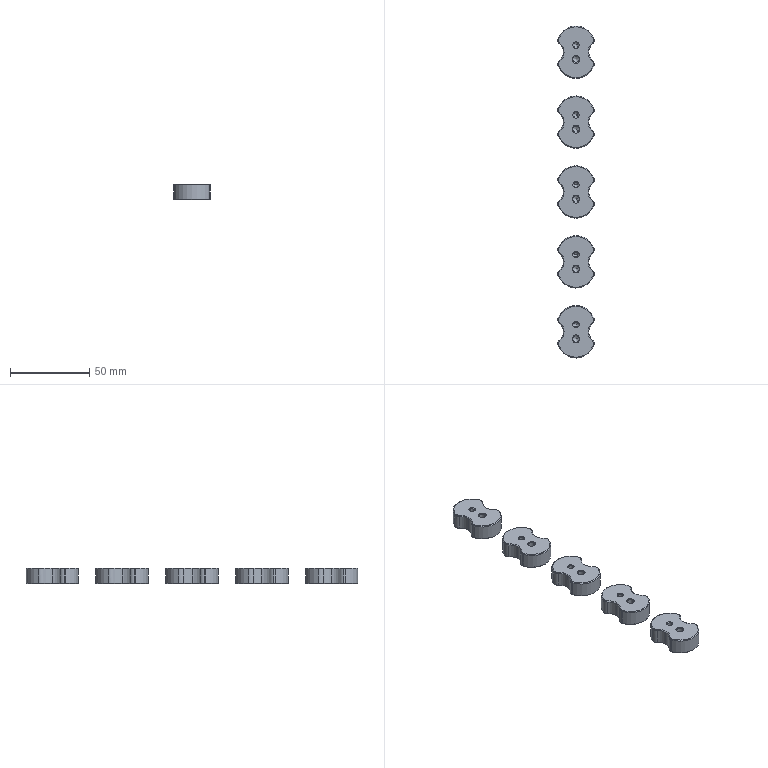NC program | NX | posted with a generic post | part box 22.923 x 209 x 10 mm
Lines 8051 to 9354 of 9354, first 1127 of 1296 lines:
(ZLEVEL_PROFILE_COPY_1_COPY , TOOL : D10JING)
N16094 T14 M6
N16096 G54
N16098 G17 G0 G90 X34.439 Y-17.238 S9500 M3
N16100 G43 Z30. H14
N16102 Z-9.
N16104 G94 G1 Z-10. F1000.
N16106 X34.352 Y-16.748
N16108 G3 X33.708 Y-15.983 R1.
N16110 G2 X33.708 Y15.983 R17. F1200.
N16112 X42.487 Y13.692 R8.
N16114 G3 X45.513 Y13.692 R2.
N16116 G2 X54.292 Y15.983 R8.
N16118 X54.292 Y-15.983 R17.
N16120 X45.513 Y-13.692 R8.
N16122 G3 X42.487 Y-13.692 R2.
N16124 G2 X33.708 Y-15.983 R8.
N16126 G3 X32.724 Y-16.158 R1.
N16128 G1 X32.313 Y-16.503
N16130 Z-9.
N16132 G0 Z53.
N16134 X-78.439 Y17.238
N16136 Z-9.
N16138 G1 Z-10. F1000.
N16140 X-78.352 Y16.748
N16142 G3 X-77.708 Y15.983 R1.
N16144 G2 X-77.708 Y-15.983 R17. F1200.
N16146 X-86.487 Y-13.692 R8.
N16148 G3 X-89.513 Y-13.692 R2.
N16150 G2 X-98.292 Y-15.983 R8.
N16152 X-98.292 Y15.983 R17.
N16154 X-89.513 Y13.692 R8.
N16156 G3 X-86.487 Y13.692 R2.
N16158 G2 X-77.708 Y15.983 R8.
N16160 G3 X-76.724 Y16.158 R1.
N16162 G1 X-76.313 Y16.503
N16164 Z-9.
N16166 G0 Z53.
N16168 X-9.561 Y-17.238
N16170 Z-9.
N16172 G1 Z-10. F1000.
N16174 X-9.648 Y-16.748
N16176 G3 X-10.292 Y-15.983 R1.
N16178 G2 X-10.292 Y15.983 R17. F1200.
N16180 X-1.513 Y13.692 R8.
N16182 G3 X1.513 Y13.692 R2.
N16184 G2 X10.292 Y15.983 R8.
N16186 X10.292 Y-15.983 R17.
N16188 X1.513 Y-13.692 R8.
N16190 G3 X-1.513 Y-13.692 R2.
N16192 G2 X-10.292 Y-15.983 R8.
N16194 G3 X-11.276 Y-16.158 R1.
N16196 G1 X-11.687 Y-16.503
N16198 Z-9.
N16200 G0 Z30.
N16202 X78.439 Y-17.238
N16204 Z-9.
N16206 G1 Z-10. F1000.
N16208 X78.352 Y-16.748
N16210 G3 X77.708 Y-15.983 R1.
N16212 G2 X77.708 Y15.983 R17. F1200.
N16214 X86.487 Y13.692 R8.
N16216 G3 X89.513 Y13.692 R2.
N16218 G2 X98.292 Y15.983 R8.
N16220 X98.292 Y-15.983 R17.
N16222 X89.513 Y-13.692 R8.
N16224 G3 X86.487 Y-13.692 R2.
N16226 G2 X77.708 Y-15.983 R8.
N16228 G3 X76.724 Y-16.158 R1.
N16230 G1 X76.313 Y-16.503
N16232 Z-9.
N16234 G0 Z53.
N16236 X-34.439 Y17.238
N16238 Z-9.
N16240 G1 Z-10. F1000.
N16242 X-34.352 Y16.748
N16244 G3 X-33.708 Y15.983 R1.
N16246 G2 X-33.708 Y-15.983 R17. F1200.
N16248 X-42.487 Y-13.692 R8.
N16250 G3 X-45.513 Y-13.692 R2.
N16252 G2 X-54.292 Y-15.983 R8.
N16254 X-54.292 Y15.983 R17.
N16256 X-45.513 Y13.692 R8.
N16258 G3 X-42.487 Y13.692 R2.
N16260 G2 X-33.708 Y15.983 R8.
N16262 G3 X-32.724 Y16.158 R1.
N16264 G1 X-32.313 Y16.503
N16266 Z-9.
N16268 G0 Z30.
N16270 M5
(HOLE_MILLING , TOOL : D2)
N16272 T17 M6
N16274 G54
N16276 G17 G0 G90 X-92.5 Y0. S9500 M3
N16278 G43 Z30. H17
N16280 Z0.5
N16282 G94 G3 X-92.95 Y-0.45 R0.45 F1150.
N16284 X-92.5 Y-0.9 R0.45
N16286 X-92.5 Y-0.9 Z0.4 I0. J0.9
N16288 X-92.5 Y-0.9 Z0.3 I0. J0.9
N16290 X-92.5 Y-0.9 Z0.2 I0. J0.9
N16292 X-92.5 Y-0.9 Z0.1 I0. J0.9
N16294 X-92.5 Y-0.9 Z0. I0. J0.9
N16296 X-92.5 Y-0.9 Z-0.1 I0. J0.9
N16298 X-92.5 Y-0.9 Z-0.2 I0. J0.9
N16300 X-92.5 Y-0.9 Z-0.3 I0. J0.9
N16302 X-92.5 Y-0.9 Z-0.4 I0. J0.9
N16304 X-92.5 Y-0.9 Z-0.5 I0. J0.9
N16306 X-92.5 Y-0.9 Z-0.6 I0. J0.9
N16308 X-92.5 Y-0.9 Z-0.7 I0. J0.9
N16310 X-92.5 Y-0.9 Z-0.8 I0. J0.9
N16312 X-92.5 Y-0.9 Z-0.9 I0. J0.9
N16314 X-92.5 Y-0.9 Z-1. I0. J0.9
N16316 X-92.5 Y-0.9 Z-1.1 I0. J0.9
N16318 X-92.5 Y-0.9 Z-1.2 I0. J0.9
N16320 X-92.5 Y-0.9 Z-1.3 I0. J0.9
N16322 X-92.5 Y-0.9 Z-1.4 I0. J0.9
N16324 X-92.5 Y-0.9 Z-1.5 I0. J0.9
N16326 X-92.5 Y-0.9 Z-1.6 I0. J0.9
N16328 X-92.5 Y-0.9 Z-1.7 I0. J0.9
N16330 X-92.5 Y-0.9 Z-1.8 I0. J0.9
N16332 X-92.5 Y-0.9 Z-1.9 I0. J0.9
N16334 X-92.5 Y-0.9 Z-2. I0. J0.9
N16336 X-92.5 Y-0.9 Z-2.1 I0. J0.9
N16338 X-92.5 Y-0.9 Z-2.2 I0. J0.9
N16340 X-92.5 Y-0.9 Z-2.3 I0. J0.9
N16342 X-92.5 Y-0.9 Z-2.4 I0. J0.9
N16344 X-92.5 Y-0.9 Z-2.5 I0. J0.9
N16346 X-92.5 Y-0.9 Z-2.6 I0. J0.9
N16348 X-92.5 Y-0.9 Z-2.7 I0. J0.9
N16350 X-92.5 Y-0.9 Z-2.8 I0. J0.9
N16352 X-92.5 Y-0.9 Z-2.9 I0. J0.9
N16354 X-92.5 Y-0.9 Z-3. I0. J0.9
N16356 X-92.5 Y-0.9 Z-3.1 I0. J0.9
N16358 X-92.5 Y-0.9 Z-3.2 I0. J0.9
N16360 X-92.5 Y-0.9 Z-3.3 I0. J0.9
N16362 X-92.5 Y-0.9 Z-3.4 I0. J0.9
N16364 X-92.5 Y-0.9 Z-3.5 I0. J0.9
N16366 X-92.5 Y-0.9 Z-3.6 I0. J0.9
N16368 X-92.5 Y-0.9 Z-3.7 I0. J0.9
N16370 X-92.5 Y-0.9 Z-3.8 I0. J0.9
N16372 X-92.5 Y-0.9 Z-3.9 I0. J0.9
N16374 X-92.5 Y-0.9 Z-4. I0. J0.9
N16376 X-92.5 Y-0.9 Z-4.1 I0. J0.9
N16378 X-92.5 Y-0.9 Z-4.2 I0. J0.9
N16380 X-92.5 Y-0.9 Z-4.3 I0. J0.9
N16382 X-92.5 Y-0.9 Z-4.4 I0. J0.9
N16384 X-92.5 Y-0.9 Z-4.5 I0. J0.9
N16386 X-92.5 Y-0.9 Z-4.6 I0. J0.9
N16388 X-92.5 Y-0.9 Z-4.7 I0. J0.9
N16390 X-92.5 Y-0.9 Z-4.8 I0. J0.9
N16392 X-92.5 Y-0.9 Z-4.9 I0. J0.9
N16394 X-92.5 Y-0.9 Z-5. I0. J0.9
N16396 X-92.5 Y-0.9 Z-5.1 I0. J0.9
N16398 X-92.5 Y-0.9 Z-5.2 I0. J0.9
N16400 X-92.5 Y-0.9 Z-5.3 I0. J0.9
N16402 X-92.5 Y-0.9 Z-5.4 I0. J0.9
N16404 X-92.5 Y-0.9 Z-5.5 I0. J0.9
N16406 X-92.5 Y-0.9 Z-5.6 I0. J0.9
N16408 X-92.5 Y-0.9 Z-5.7 I0. J0.9
N16410 X-92.5 Y-0.9 Z-5.8 I0. J0.9
N16412 X-92.5 Y-0.9 Z-5.9 I0. J0.9
N16414 X-92.5 Y-0.9 Z-6. I0. J0.9
N16416 X-92.5 Y-0.9 Z-6.1 I0. J0.9
N16418 X-92.5 Y-0.9 Z-6.2 I0. J0.9
N16420 X-92.5 Y-0.9 Z-6.3 I0. J0.9
N16422 X-92.5 Y-0.9 Z-6.4 I0. J0.9
N16424 X-92.5 Y-0.9 Z-6.5 I0. J0.9
N16426 X-92.5 Y-0.9 Z-6.6 I0. J0.9
N16428 X-92.5 Y-0.9 Z-6.7 I0. J0.9
N16430 X-92.5 Y-0.9 Z-6.8 I0. J0.9
N16432 X-92.5 Y-0.9 Z-6.9 I0. J0.9
N16434 X-92.5 Y-0.9 Z-7. I0. J0.9
N16436 X-91.6 Y0. R0.9
N16438 X-92.5 Y-0.9 R-0.9
N16440 X-92.05 Y-0.45 R0.45
N16442 X-92.5 Y0. R0.45
N16444 G0 Z30.
N16446 X-83.5
N16448 Z0.5
N16450 G3 X-83.7 Y-0.2 R0.2
N16452 X-83.5 Y-0.4 R0.2
N16454 X-83.5 Y-0.4 Z0.4 I0. J0.4
N16456 X-83.5 Y-0.4 Z0.3 I0. J0.4
N16458 X-83.5 Y-0.4 Z0.2 I0. J0.4
N16460 X-83.5 Y-0.4 Z0.1 I0. J0.4
N16462 X-83.5 Y-0.4 Z0. I0. J0.4
N16464 X-83.5 Y-0.4 Z-0.1 I0. J0.4
N16466 X-83.5 Y-0.4 Z-0.2 I0. J0.4
N16468 X-83.5 Y-0.4 Z-0.3 I0. J0.4
N16470 X-83.5 Y-0.4 Z-0.4 I0. J0.4
N16472 X-83.5 Y-0.4 Z-0.5 I0. J0.4
N16474 X-83.5 Y-0.4 Z-0.6 I0. J0.4
N16476 X-83.5 Y-0.4 Z-0.7 I0. J0.4
N16478 X-83.5 Y-0.4 Z-0.8 I0. J0.4
N16480 X-83.5 Y-0.4 Z-0.9 I0. J0.4
N16482 X-83.5 Y-0.4 Z-1. I0. J0.4
N16484 X-83.5 Y-0.4 Z-1.1 I0. J0.4
N16486 X-83.5 Y-0.4 Z-1.2 I0. J0.4
N16488 X-83.5 Y-0.4 Z-1.3 I0. J0.4
N16490 X-83.5 Y-0.4 Z-1.4 I0. J0.4
N16492 X-83.5 Y-0.4 Z-1.5 I0. J0.4
N16494 X-83.5 Y-0.4 Z-1.6 I0. J0.4
N16496 X-83.5 Y-0.4 Z-1.7 I0. J0.4
N16498 X-83.5 Y-0.4 Z-1.8 I0. J0.4
N16500 X-83.5 Y-0.4 Z-1.9 I0. J0.4
N16502 X-83.5 Y-0.4 Z-2. I0. J0.4
N16504 X-83.5 Y-0.4 Z-2.1 I0. J0.4
N16506 X-83.5 Y-0.4 Z-2.2 I0. J0.4
N16508 X-83.5 Y-0.4 Z-2.3 I0. J0.4
N16510 X-83.5 Y-0.4 Z-2.4 I0. J0.4
N16512 X-83.5 Y-0.4 Z-2.5 I0. J0.4
N16514 X-83.5 Y-0.4 Z-2.6 I0. J0.4
N16516 X-83.5 Y-0.4 Z-2.7 I0. J0.4
N16518 X-83.5 Y-0.4 Z-2.8 I0. J0.4
N16520 X-83.5 Y-0.4 Z-2.9 I0. J0.4
N16522 X-83.5 Y-0.4 Z-3. I0. J0.4
N16524 X-83.5 Y-0.4 Z-3.1 I0. J0.4
N16526 X-83.5 Y-0.4 Z-3.2 I0. J0.4
N16528 X-83.5 Y-0.4 Z-3.3 I0. J0.4
N16530 X-83.5 Y-0.4 Z-3.4 I0. J0.4
N16532 X-83.5 Y-0.4 Z-3.5 I0. J0.4
N16534 X-83.5 Y-0.4 Z-3.6 I0. J0.4
N16536 X-83.5 Y-0.4 Z-3.7 I0. J0.4
N16538 X-83.5 Y-0.4 Z-3.8 I0. J0.4
N16540 X-83.5 Y-0.4 Z-3.9 I0. J0.4
N16542 X-83.5 Y-0.4 Z-4. I0. J0.4
N16544 X-83.5 Y-0.4 Z-4.1 I0. J0.4
N16546 X-83.5 Y-0.4 Z-4.2 I0. J0.4
N16548 X-83.5 Y-0.4 Z-4.3 I0. J0.4
N16550 X-83.5 Y-0.4 Z-4.4 I0. J0.4
N16552 X-83.5 Y-0.4 Z-4.5 I0. J0.4
N16554 X-83.5 Y-0.4 Z-4.6 I0. J0.4
N16556 X-83.5 Y-0.4 Z-4.7 I0. J0.4
N16558 X-83.5 Y-0.4 Z-4.8 I0. J0.4
N16560 X-83.5 Y-0.4 Z-4.9 I0. J0.4
N16562 X-83.5 Y-0.4 Z-5. I0. J0.4
N16564 X-83.5 Y-0.4 Z-5.1 I0. J0.4
N16566 X-83.5 Y-0.4 Z-5.2 I0. J0.4
N16568 X-83.5 Y-0.4 Z-5.3 I0. J0.4
N16570 X-83.5 Y-0.4 Z-5.4 I0. J0.4
N16572 X-83.5 Y-0.4 Z-5.5 I0. J0.4
N16574 X-83.5 Y-0.4 Z-5.6 I0. J0.4
N16576 X-83.5 Y-0.4 Z-5.7 I0. J0.4
N16578 X-83.5 Y-0.4 Z-5.8 I0. J0.4
N16580 X-83.5 Y-0.4 Z-5.9 I0. J0.4
N16582 X-83.5 Y-0.4 Z-6. I0. J0.4
N16584 X-83.5 Y-0.4 Z-6.1 I0. J0.4
N16586 X-83.5 Y-0.4 Z-6.2 I0. J0.4
N16588 X-83.5 Y-0.4 Z-6.3 I0. J0.4
N16590 X-83.5 Y-0.4 Z-6.4 I0. J0.4
N16592 X-83.5 Y-0.4 Z-6.5 I0. J0.4
N16594 X-83.5 Y-0.4 Z-6.6 I0. J0.4
N16596 X-83.5 Y-0.4 Z-6.7 I0. J0.4
N16598 X-83.5 Y-0.4 Z-6.8 I0. J0.4
N16600 X-83.5 Y-0.4 Z-6.9 I0. J0.4
N16602 X-83.5 Y-0.4 Z-7. I0. J0.4
N16604 X-83.1 Y0. R0.4
N16606 X-83.5 Y-0.4 R-0.4
N16608 X-83.3 Y-0.2 R0.2
N16610 X-83.5 Y0. R0.2
N16612 G0 Z30.
N16614 X-48.5
N16616 Z0.5
N16618 G3 X-48.95 Y-0.45 R0.45
N16620 X-48.5 Y-0.9 R0.45
N16622 X-48.5 Y-0.9 Z0.4 I0. J0.9
N16624 X-48.5 Y-0.9 Z0.3 I0. J0.9
N16626 X-48.5 Y-0.9 Z0.2 I0. J0.9
N16628 X-48.5 Y-0.9 Z0.1 I0. J0.9
N16630 X-48.5 Y-0.9 Z0. I0. J0.9
N16632 X-48.5 Y-0.9 Z-0.1 I0. J0.9
N16634 X-48.5 Y-0.9 Z-0.2 I0. J0.9
N16636 X-48.5 Y-0.9 Z-0.3 I0. J0.9
N16638 X-48.5 Y-0.9 Z-0.4 I0. J0.9
N16640 X-48.5 Y-0.9 Z-0.5 I0. J0.9
N16642 X-48.5 Y-0.9 Z-0.6 I0. J0.9
N16644 X-48.5 Y-0.9 Z-0.7 I0. J0.9
N16646 X-48.5 Y-0.9 Z-0.8 I0. J0.9
N16648 X-48.5 Y-0.9 Z-0.9 I0. J0.9
N16650 X-48.5 Y-0.9 Z-1. I0. J0.9
N16652 X-48.5 Y-0.9 Z-1.1 I0. J0.9
N16654 X-48.5 Y-0.9 Z-1.2 I0. J0.9
N16656 X-48.5 Y-0.9 Z-1.3 I0. J0.9
N16658 X-48.5 Y-0.9 Z-1.4 I0. J0.9
N16660 X-48.5 Y-0.9 Z-1.5 I0. J0.9
N16662 X-48.5 Y-0.9 Z-1.6 I0. J0.9
N16664 X-48.5 Y-0.9 Z-1.7 I0. J0.9
N16666 X-48.5 Y-0.9 Z-1.8 I0. J0.9
N16668 X-48.5 Y-0.9 Z-1.9 I0. J0.9
N16670 X-48.5 Y-0.9 Z-2. I0. J0.9
N16672 X-48.5 Y-0.9 Z-2.1 I0. J0.9
N16674 X-48.5 Y-0.9 Z-2.2 I0. J0.9
N16676 X-48.5 Y-0.9 Z-2.3 I0. J0.9
N16678 X-48.5 Y-0.9 Z-2.4 I0. J0.9
N16680 X-48.5 Y-0.9 Z-2.5 I0. J0.9
N16682 X-48.5 Y-0.9 Z-2.6 I0. J0.9
N16684 X-48.5 Y-0.9 Z-2.7 I0. J0.9
N16686 X-48.5 Y-0.9 Z-2.8 I0. J0.9
N16688 X-48.5 Y-0.9 Z-2.9 I0. J0.9
N16690 X-48.5 Y-0.9 Z-3. I0. J0.9
N16692 X-48.5 Y-0.9 Z-3.1 I0. J0.9
N16694 X-48.5 Y-0.9 Z-3.2 I0. J0.9
N16696 X-48.5 Y-0.9 Z-3.3 I0. J0.9
N16698 X-48.5 Y-0.9 Z-3.4 I0. J0.9
N16700 X-48.5 Y-0.9 Z-3.5 I0. J0.9
N16702 X-48.5 Y-0.9 Z-3.6 I0. J0.9
N16704 X-48.5 Y-0.9 Z-3.7 I0. J0.9
N16706 X-48.5 Y-0.9 Z-3.8 I0. J0.9
N16708 X-48.5 Y-0.9 Z-3.9 I0. J0.9
N16710 X-48.5 Y-0.9 Z-4. I0. J0.9
N16712 X-48.5 Y-0.9 Z-4.1 I0. J0.9
N16714 X-48.5 Y-0.9 Z-4.2 I0. J0.9
N16716 X-48.5 Y-0.9 Z-4.3 I0. J0.9
N16718 X-48.5 Y-0.9 Z-4.4 I0. J0.9
N16720 X-48.5 Y-0.9 Z-4.5 I0. J0.9
N16722 X-48.5 Y-0.9 Z-4.6 I0. J0.9
N16724 X-48.5 Y-0.9 Z-4.7 I0. J0.9
N16726 X-48.5 Y-0.9 Z-4.8 I0. J0.9
N16728 X-48.5 Y-0.9 Z-4.9 I0. J0.9
N16730 X-48.5 Y-0.9 Z-5. I0. J0.9
N16732 X-48.5 Y-0.9 Z-5.1 I0. J0.9
N16734 X-48.5 Y-0.9 Z-5.2 I0. J0.9
N16736 X-48.5 Y-0.9 Z-5.3 I0. J0.9
N16738 X-48.5 Y-0.9 Z-5.4 I0. J0.9
N16740 X-48.5 Y-0.9 Z-5.5 I0. J0.9
N16742 X-48.5 Y-0.9 Z-5.6 I0. J0.9
N16744 X-48.5 Y-0.9 Z-5.7 I0. J0.9
N16746 X-48.5 Y-0.9 Z-5.8 I0. J0.9
N16748 X-48.5 Y-0.9 Z-5.9 I0. J0.9
N16750 X-48.5 Y-0.9 Z-6. I0. J0.9
N16752 X-48.5 Y-0.9 Z-6.1 I0. J0.9
N16754 X-48.5 Y-0.9 Z-6.2 I0. J0.9
N16756 X-48.5 Y-0.9 Z-6.3 I0. J0.9
N16758 X-48.5 Y-0.9 Z-6.4 I0. J0.9
N16760 X-48.5 Y-0.9 Z-6.5 I0. J0.9
N16762 X-48.5 Y-0.9 Z-6.6 I0. J0.9
N16764 X-48.5 Y-0.9 Z-6.7 I0. J0.9
N16766 X-48.5 Y-0.9 Z-6.8 I0. J0.9
N16768 X-48.5 Y-0.9 Z-6.9 I0. J0.9
N16770 X-48.5 Y-0.9 Z-7. I0. J0.9
N16772 X-47.6 Y0. R0.9
N16774 X-48.5 Y-0.9 R-0.9
N16776 X-48.05 Y-0.45 R0.45
N16778 X-48.5 Y0. R0.45
N16780 G0 Z30.
N16782 X-39.5
N16784 Z0.5
N16786 G3 X-39.7 Y-0.2 R0.2
N16788 X-39.5 Y-0.4 R0.2
N16790 X-39.5 Y-0.4 Z0.4 I0. J0.4
N16792 X-39.5 Y-0.4 Z0.3 I0. J0.4
N16794 X-39.5 Y-0.4 Z0.2 I0. J0.4
N16796 X-39.5 Y-0.4 Z0.1 I0. J0.4
N16798 X-39.5 Y-0.4 Z0. I0. J0.4
N16800 X-39.5 Y-0.4 Z-0.1 I0. J0.4
N16802 X-39.5 Y-0.4 Z-0.2 I0. J0.4
N16804 X-39.5 Y-0.4 Z-0.3 I0. J0.4
N16806 X-39.5 Y-0.4 Z-0.4 I0. J0.4
N16808 X-39.5 Y-0.4 Z-0.5 I0. J0.4
N16810 X-39.5 Y-0.4 Z-0.6 I0. J0.4
N16812 X-39.5 Y-0.4 Z-0.7 I0. J0.4
N16814 X-39.5 Y-0.4 Z-0.8 I0. J0.4
N16816 X-39.5 Y-0.4 Z-0.9 I0. J0.4
N16818 X-39.5 Y-0.4 Z-1. I0. J0.4
N16820 X-39.5 Y-0.4 Z-1.1 I0. J0.4
N16822 X-39.5 Y-0.4 Z-1.2 I0. J0.4
N16824 X-39.5 Y-0.4 Z-1.3 I0. J0.4
N16826 X-39.5 Y-0.4 Z-1.4 I0. J0.4
N16828 X-39.5 Y-0.4 Z-1.5 I0. J0.4
N16830 X-39.5 Y-0.4 Z-1.6 I0. J0.4
N16832 X-39.5 Y-0.4 Z-1.7 I0. J0.4
N16834 X-39.5 Y-0.4 Z-1.8 I0. J0.4
N16836 X-39.5 Y-0.4 Z-1.9 I0. J0.4
N16838 X-39.5 Y-0.4 Z-2. I0. J0.4
N16840 X-39.5 Y-0.4 Z-2.1 I0. J0.4
N16842 X-39.5 Y-0.4 Z-2.2 I0. J0.4
N16844 X-39.5 Y-0.4 Z-2.3 I0. J0.4
N16846 X-39.5 Y-0.4 Z-2.4 I0. J0.4
N16848 X-39.5 Y-0.4 Z-2.5 I0. J0.4
N16850 X-39.5 Y-0.4 Z-2.6 I0. J0.4
N16852 X-39.5 Y-0.4 Z-2.7 I0. J0.4
N16854 X-39.5 Y-0.4 Z-2.8 I0. J0.4
N16856 X-39.5 Y-0.4 Z-2.9 I0. J0.4
N16858 X-39.5 Y-0.4 Z-3. I0. J0.4
N16860 X-39.5 Y-0.4 Z-3.1 I0. J0.4
N16862 X-39.5 Y-0.4 Z-3.2 I0. J0.4
N16864 X-39.5 Y-0.4 Z-3.3 I0. J0.4
N16866 X-39.5 Y-0.4 Z-3.4 I0. J0.4
N16868 X-39.5 Y-0.4 Z-3.5 I0. J0.4
N16870 X-39.5 Y-0.4 Z-3.6 I0. J0.4
N16872 X-39.5 Y-0.4 Z-3.7 I0. J0.4
N16874 X-39.5 Y-0.4 Z-3.8 I0. J0.4
N16876 X-39.5 Y-0.4 Z-3.9 I0. J0.4
N16878 X-39.5 Y-0.4 Z-4. I0. J0.4
N16880 X-39.5 Y-0.4 Z-4.1 I0. J0.4
N16882 X-39.5 Y-0.4 Z-4.2 I0. J0.4
N16884 X-39.5 Y-0.4 Z-4.3 I0. J0.4
N16886 X-39.5 Y-0.4 Z-4.4 I0. J0.4
N16888 X-39.5 Y-0.4 Z-4.5 I0. J0.4
N16890 X-39.5 Y-0.4 Z-4.6 I0. J0.4
N16892 X-39.5 Y-0.4 Z-4.7 I0. J0.4
N16894 X-39.5 Y-0.4 Z-4.8 I0. J0.4
N16896 X-39.5 Y-0.4 Z-4.9 I0. J0.4
N16898 X-39.5 Y-0.4 Z-5. I0. J0.4
N16900 X-39.5 Y-0.4 Z-5.1 I0. J0.4
N16902 X-39.5 Y-0.4 Z-5.2 I0. J0.4
N16904 X-39.5 Y-0.4 Z-5.3 I0. J0.4
N16906 X-39.5 Y-0.4 Z-5.4 I0. J0.4
N16908 X-39.5 Y-0.4 Z-5.5 I0. J0.4
N16910 X-39.5 Y-0.4 Z-5.6 I0. J0.4
N16912 X-39.5 Y-0.4 Z-5.7 I0. J0.4
N16914 X-39.5 Y-0.4 Z-5.8 I0. J0.4
N16916 X-39.5 Y-0.4 Z-5.9 I0. J0.4
N16918 X-39.5 Y-0.4 Z-6. I0. J0.4
N16920 X-39.5 Y-0.4 Z-6.1 I0. J0.4
N16922 X-39.5 Y-0.4 Z-6.2 I0. J0.4
N16924 X-39.5 Y-0.4 Z-6.3 I0. J0.4
N16926 X-39.5 Y-0.4 Z-6.4 I0. J0.4
N16928 X-39.5 Y-0.4 Z-6.5 I0. J0.4
N16930 X-39.5 Y-0.4 Z-6.6 I0. J0.4
N16932 X-39.5 Y-0.4 Z-6.7 I0. J0.4
N16934 X-39.5 Y-0.4 Z-6.8 I0. J0.4
N16936 X-39.5 Y-0.4 Z-6.9 I0. J0.4
N16938 X-39.5 Y-0.4 Z-7. I0. J0.4
N16940 X-39.1 Y0. R0.4
N16942 X-39.5 Y-0.4 R-0.4
N16944 X-39.3 Y-0.2 R0.2
N16946 X-39.5 Y0. R0.2
N16948 G0 Z30.
N16950 X-4.5
N16952 Z0.5
N16954 G3 X-4.95 Y-0.45 R0.45
N16956 X-4.5 Y-0.9 R0.45
N16958 X-4.5 Y-0.9 Z0.4 I0. J0.9
N16960 X-4.5 Y-0.9 Z0.3 I0. J0.9
N16962 X-4.5 Y-0.9 Z0.2 I0. J0.9
N16964 X-4.5 Y-0.9 Z0.1 I0. J0.9
N16966 X-4.5 Y-0.9 Z0. I0. J0.9
N16968 X-4.5 Y-0.9 Z-0.1 I0. J0.9
N16970 X-4.5 Y-0.9 Z-0.2 I0. J0.9
N16972 X-4.5 Y-0.9 Z-0.3 I0. J0.9
N16974 X-4.5 Y-0.9 Z-0.4 I0. J0.9
N16976 X-4.5 Y-0.9 Z-0.5 I0. J0.9
N16978 X-4.5 Y-0.9 Z-0.6 I0. J0.9
N16980 X-4.5 Y-0.9 Z-0.7 I0. J0.9
N16982 X-4.5 Y-0.9 Z-0.8 I0. J0.9
N16984 X-4.5 Y-0.9 Z-0.9 I0. J0.9
N16986 X-4.5 Y-0.9 Z-1. I0. J0.9
N16988 X-4.5 Y-0.9 Z-1.1 I0. J0.9
N16990 X-4.5 Y-0.9 Z-1.2 I0. J0.9
N16992 X-4.5 Y-0.9 Z-1.3 I0. J0.9
N16994 X-4.5 Y-0.9 Z-1.4 I0. J0.9
N16996 X-4.5 Y-0.9 Z-1.5 I0. J0.9
N16998 X-4.5 Y-0.9 Z-1.6 I0. J0.9
N17000 X-4.5 Y-0.9 Z-1.7 I0. J0.9
N17002 X-4.5 Y-0.9 Z-1.8 I0. J0.9
N17004 X-4.5 Y-0.9 Z-1.9 I0. J0.9
N17006 X-4.5 Y-0.9 Z-2. I0. J0.9
N17008 X-4.5 Y-0.9 Z-2.1 I0. J0.9
N17010 X-4.5 Y-0.9 Z-2.2 I0. J0.9
N17012 X-4.5 Y-0.9 Z-2.3 I0. J0.9
N17014 X-4.5 Y-0.9 Z-2.4 I0. J0.9
N17016 X-4.5 Y-0.9 Z-2.5 I0. J0.9
N17018 X-4.5 Y-0.9 Z-2.6 I0. J0.9
N17020 X-4.5 Y-0.9 Z-2.7 I0. J0.9
N17022 X-4.5 Y-0.9 Z-2.8 I0. J0.9
N17024 X-4.5 Y-0.9 Z-2.9 I0. J0.9
N17026 X-4.5 Y-0.9 Z-3. I0. J0.9
N17028 X-4.5 Y-0.9 Z-3.1 I0. J0.9
N17030 X-4.5 Y-0.9 Z-3.2 I0. J0.9
N17032 X-4.5 Y-0.9 Z-3.3 I0. J0.9
N17034 X-4.5 Y-0.9 Z-3.4 I0. J0.9
N17036 X-4.5 Y-0.9 Z-3.5 I0. J0.9
N17038 X-4.5 Y-0.9 Z-3.6 I0. J0.9
N17040 X-4.5 Y-0.9 Z-3.7 I0. J0.9
N17042 X-4.5 Y-0.9 Z-3.8 I0. J0.9
N17044 X-4.5 Y-0.9 Z-3.9 I0. J0.9
N17046 X-4.5 Y-0.9 Z-4. I0. J0.9
N17048 X-4.5 Y-0.9 Z-4.1 I0. J0.9
N17050 X-4.5 Y-0.9 Z-4.2 I0. J0.9
N17052 X-4.5 Y-0.9 Z-4.3 I0. J0.9
N17054 X-4.5 Y-0.9 Z-4.4 I0. J0.9
N17056 X-4.5 Y-0.9 Z-4.5 I0. J0.9
N17058 X-4.5 Y-0.9 Z-4.6 I0. J0.9
N17060 X-4.5 Y-0.9 Z-4.7 I0. J0.9
N17062 X-4.5 Y-0.9 Z-4.8 I0. J0.9
N17064 X-4.5 Y-0.9 Z-4.9 I0. J0.9
N17066 X-4.5 Y-0.9 Z-5. I0. J0.9
N17068 X-4.5 Y-0.9 Z-5.1 I0. J0.9
N17070 X-4.5 Y-0.9 Z-5.2 I0. J0.9
N17072 X-4.5 Y-0.9 Z-5.3 I0. J0.9
N17074 X-4.5 Y-0.9 Z-5.4 I0. J0.9
N17076 X-4.5 Y-0.9 Z-5.5 I0. J0.9
N17078 X-4.5 Y-0.9 Z-5.6 I0. J0.9
N17080 X-4.5 Y-0.9 Z-5.7 I0. J0.9
N17082 X-4.5 Y-0.9 Z-5.8 I0. J0.9
N17084 X-4.5 Y-0.9 Z-5.9 I0. J0.9
N17086 X-4.5 Y-0.9 Z-6. I0. J0.9
N17088 X-4.5 Y-0.9 Z-6.1 I0. J0.9
N17090 X-4.5 Y-0.9 Z-6.2 I0. J0.9
N17092 X-4.5 Y-0.9 Z-6.3 I0. J0.9
N17094 X-4.5 Y-0.9 Z-6.4 I0. J0.9
N17096 X-4.5 Y-0.9 Z-6.5 I0. J0.9
N17098 X-4.5 Y-0.9 Z-6.6 I0. J0.9
N17100 X-4.5 Y-0.9 Z-6.7 I0. J0.9
N17102 X-4.5 Y-0.9 Z-6.8 I0. J0.9
N17104 X-4.5 Y-0.9 Z-6.9 I0. J0.9
N17106 X-4.5 Y-0.9 Z-7. I0. J0.9
N17108 X-3.6 Y0. R0.9
N17110 X-4.5 Y-0.9 R-0.9
N17112 X-4.05 Y-0.45 R0.45
N17114 X-4.5 Y0. R0.45
N17116 G0 Z30.
N17118 X4.5
N17120 Z0.5
N17122 G3 X4.3 Y-0.2 R0.2
N17124 X4.5 Y-0.4 R0.2
N17126 X4.5 Y-0.4 Z0.4 I0. J0.4
N17128 X4.5 Y-0.4 Z0.3 I0. J0.4
N17130 X4.5 Y-0.4 Z0.2 I0. J0.4
N17132 X4.5 Y-0.4 Z0.1 I0. J0.4
N17134 X4.5 Y-0.4 Z0. I0. J0.4
N17136 X4.5 Y-0.4 Z-0.1 I0. J0.4
N17138 X4.5 Y-0.4 Z-0.2 I0. J0.4
N17140 X4.5 Y-0.4 Z-0.3 I0. J0.4
N17142 X4.5 Y-0.4 Z-0.4 I0. J0.4
N17144 X4.5 Y-0.4 Z-0.5 I0. J0.4
N17146 X4.5 Y-0.4 Z-0.6 I0. J0.4
N17148 X4.5 Y-0.4 Z-0.7 I0. J0.4
N17150 X4.5 Y-0.4 Z-0.8 I0. J0.4
N17152 X4.5 Y-0.4 Z-0.9 I0. J0.4
N17154 X4.5 Y-0.4 Z-1. I0. J0.4
N17156 X4.5 Y-0.4 Z-1.1 I0. J0.4
N17158 X4.5 Y-0.4 Z-1.2 I0. J0.4
N17160 X4.5 Y-0.4 Z-1.3 I0. J0.4
N17162 X4.5 Y-0.4 Z-1.4 I0. J0.4
N17164 X4.5 Y-0.4 Z-1.5 I0. J0.4
N17166 X4.5 Y-0.4 Z-1.6 I0. J0.4
N17168 X4.5 Y-0.4 Z-1.7 I0. J0.4
N17170 X4.5 Y-0.4 Z-1.8 I0. J0.4
N17172 X4.5 Y-0.4 Z-1.9 I0. J0.4
N17174 X4.5 Y-0.4 Z-2. I0. J0.4
N17176 X4.5 Y-0.4 Z-2.1 I0. J0.4
N17178 X4.5 Y-0.4 Z-2.2 I0. J0.4
N17180 X4.5 Y-0.4 Z-2.3 I0. J0.4
N17182 X4.5 Y-0.4 Z-2.4 I0. J0.4
N17184 X4.5 Y-0.4 Z-2.5 I0. J0.4
N17186 X4.5 Y-0.4 Z-2.6 I0. J0.4
N17188 X4.5 Y-0.4 Z-2.7 I0. J0.4
N17190 X4.5 Y-0.4 Z-2.8 I0. J0.4
N17192 X4.5 Y-0.4 Z-2.9 I0. J0.4
N17194 X4.5 Y-0.4 Z-3. I0. J0.4
N17196 X4.5 Y-0.4 Z-3.1 I0. J0.4
N17198 X4.5 Y-0.4 Z-3.2 I0. J0.4
N17200 X4.5 Y-0.4 Z-3.3 I0. J0.4
N17202 X4.5 Y-0.4 Z-3.4 I0. J0.4
N17204 X4.5 Y-0.4 Z-3.5 I0. J0.4
N17206 X4.5 Y-0.4 Z-3.6 I0. J0.4
N17208 X4.5 Y-0.4 Z-3.7 I0. J0.4
N17210 X4.5 Y-0.4 Z-3.8 I0. J0.4
N17212 X4.5 Y-0.4 Z-3.9 I0. J0.4
N17214 X4.5 Y-0.4 Z-4. I0. J0.4
N17216 X4.5 Y-0.4 Z-4.1 I0. J0.4
N17218 X4.5 Y-0.4 Z-4.2 I0. J0.4
N17220 X4.5 Y-0.4 Z-4.3 I0. J0.4
N17222 X4.5 Y-0.4 Z-4.4 I0. J0.4
N17224 X4.5 Y-0.4 Z-4.5 I0. J0.4
N17226 X4.5 Y-0.4 Z-4.6 I0. J0.4
N17228 X4.5 Y-0.4 Z-4.7 I0. J0.4
N17230 X4.5 Y-0.4 Z-4.8 I0. J0.4
N17232 X4.5 Y-0.4 Z-4.9 I0. J0.4
N17234 X4.5 Y-0.4 Z-5. I0. J0.4
N17236 X4.5 Y-0.4 Z-5.1 I0. J0.4
N17238 X4.5 Y-0.4 Z-5.2 I0. J0.4
N17240 X4.5 Y-0.4 Z-5.3 I0. J0.4
N17242 X4.5 Y-0.4 Z-5.4 I0. J0.4
N17244 X4.5 Y-0.4 Z-5.5 I0. J0.4
N17246 X4.5 Y-0.4 Z-5.6 I0. J0.4
N17248 X4.5 Y-0.4 Z-5.7 I0. J0.4
N17250 X4.5 Y-0.4 Z-5.8 I0. J0.4
N17252 X4.5 Y-0.4 Z-5.9 I0. J0.4
N17254 X4.5 Y-0.4 Z-6. I0. J0.4
N17256 X4.5 Y-0.4 Z-6.1 I0. J0.4
N17258 X4.5 Y-0.4 Z-6.2 I0. J0.4
N17260 X4.5 Y-0.4 Z-6.3 I0. J0.4
N17262 X4.5 Y-0.4 Z-6.4 I0. J0.4
N17264 X4.5 Y-0.4 Z-6.5 I0. J0.4
N17266 X4.5 Y-0.4 Z-6.6 I0. J0.4
N17268 X4.5 Y-0.4 Z-6.7 I0. J0.4
N17270 X4.5 Y-0.4 Z-6.8 I0. J0.4
N17272 X4.5 Y-0.4 Z-6.9 I0. J0.4
N17274 X4.5 Y-0.4 Z-7. I0. J0.4
N17276 X4.9 Y0. R0.4
N17278 X4.5 Y-0.4 R-0.4
N17280 X4.7 Y-0.2 R0.2
N17282 X4.5 Y0. R0.2
N17284 G0 Z30.
N17286 X39.5
N17288 Z0.5
N17290 G3 X39.05 Y-0.45 R0.45
N17292 X39.5 Y-0.9 R0.45
N17294 X39.5 Y-0.9 Z0.4 I0. J0.9
N17296 X39.5 Y-0.9 Z0.3 I0. J0.9
N17298 X39.5 Y-0.9 Z0.2 I0. J0.9
N17300 X39.5 Y-0.9 Z0.1 I0. J0.9
N17302 X39.5 Y-0.9 Z0. I0. J0.9
N17304 X39.5 Y-0.9 Z-0.1 I0. J0.9
N17306 X39.5 Y-0.9 Z-0.2 I0. J0.9
N17308 X39.5 Y-0.9 Z-0.3 I0. J0.9
N17310 X39.5 Y-0.9 Z-0.4 I0. J0.9
N17312 X39.5 Y-0.9 Z-0.5 I0. J0.9
N17314 X39.5 Y-0.9 Z-0.6 I0. J0.9
N17316 X39.5 Y-0.9 Z-0.7 I0. J0.9
N17318 X39.5 Y-0.9 Z-0.8 I0. J0.9
N17320 X39.5 Y-0.9 Z-0.9 I0. J0.9
N17322 X39.5 Y-0.9 Z-1. I0. J0.9
N17324 X39.5 Y-0.9 Z-1.1 I0. J0.9
N17326 X39.5 Y-0.9 Z-1.2 I0. J0.9
N17328 X39.5 Y-0.9 Z-1.3 I0. J0.9
N17330 X39.5 Y-0.9 Z-1.4 I0. J0.9
N17332 X39.5 Y-0.9 Z-1.5 I0. J0.9
N17334 X39.5 Y-0.9 Z-1.6 I0. J0.9
N17336 X39.5 Y-0.9 Z-1.7 I0. J0.9
N17338 X39.5 Y-0.9 Z-1.8 I0. J0.9
N17340 X39.5 Y-0.9 Z-1.9 I0. J0.9
N17342 X39.5 Y-0.9 Z-2. I0. J0.9
N17344 X39.5 Y-0.9 Z-2.1 I0. J0.9
N17346 X39.5 Y-0.9 Z-2.2 I0. J0.9
N17348 X39.5 Y-0.9 Z-2.3 I0. J0.9
N17350 X39.5 Y-0.9 Z-2.4 I0. J0.9
N17352 X39.5 Y-0.9 Z-2.5 I0. J0.9
N17354 X39.5 Y-0.9 Z-2.6 I0. J0.9
N17356 X39.5 Y-0.9 Z-2.7 I0. J0.9
N17358 X39.5 Y-0.9 Z-2.8 I0. J0.9
N17360 X39.5 Y-0.9 Z-2.9 I0. J0.9
N17362 X39.5 Y-0.9 Z-3. I0. J0.9
N17364 X39.5 Y-0.9 Z-3.1 I0. J0.9
N17366 X39.5 Y-0.9 Z-3.2 I0. J0.9
N17368 X39.5 Y-0.9 Z-3.3 I0. J0.9
N17370 X39.5 Y-0.9 Z-3.4 I0. J0.9
N17372 X39.5 Y-0.9 Z-3.5 I0. J0.9
N17374 X39.5 Y-0.9 Z-3.6 I0. J0.9
N17376 X39.5 Y-0.9 Z-3.7 I0. J0.9
N17378 X39.5 Y-0.9 Z-3.8 I0. J0.9
N17380 X39.5 Y-0.9 Z-3.9 I0. J0.9
N17382 X39.5 Y-0.9 Z-4. I0. J0.9
N17384 X39.5 Y-0.9 Z-4.1 I0. J0.9
N17386 X39.5 Y-0.9 Z-4.2 I0. J0.9
N17388 X39.5 Y-0.9 Z-4.3 I0. J0.9
N17390 X39.5 Y-0.9 Z-4.4 I0. J0.9
N17392 X39.5 Y-0.9 Z-4.5 I0. J0.9
N17394 X39.5 Y-0.9 Z-4.6 I0. J0.9
N17396 X39.5 Y-0.9 Z-4.7 I0. J0.9
N17398 X39.5 Y-0.9 Z-4.8 I0. J0.9
N17400 X39.5 Y-0.9 Z-4.9 I0. J0.9
N17402 X39.5 Y-0.9 Z-5. I0. J0.9
N17404 X39.5 Y-0.9 Z-5.1 I0. J0.9
N17406 X39.5 Y-0.9 Z-5.2 I0. J0.9
N17408 X39.5 Y-0.9 Z-5.3 I0. J0.9
N17410 X39.5 Y-0.9 Z-5.4 I0. J0.9
N17412 X39.5 Y-0.9 Z-5.5 I0. J0.9
N17414 X39.5 Y-0.9 Z-5.6 I0. J0.9
N17416 X39.5 Y-0.9 Z-5.7 I0. J0.9
N17418 X39.5 Y-0.9 Z-5.8 I0. J0.9
N17420 X39.5 Y-0.9 Z-5.9 I0. J0.9
N17422 X39.5 Y-0.9 Z-6. I0. J0.9
N17424 X39.5 Y-0.9 Z-6.1 I0. J0.9
N17426 X39.5 Y-0.9 Z-6.2 I0. J0.9
N17428 X39.5 Y-0.9 Z-6.3 I0. J0.9
N17430 X39.5 Y-0.9 Z-6.4 I0. J0.9
N17432 X39.5 Y-0.9 Z-6.5 I0. J0.9
N17434 X39.5 Y-0.9 Z-6.6 I0. J0.9
N17436 X39.5 Y-0.9 Z-6.7 I0. J0.9
N17438 X39.5 Y-0.9 Z-6.8 I0. J0.9
N17440 X39.5 Y-0.9 Z-6.9 I0. J0.9
N17442 X39.5 Y-0.9 Z-7. I0. J0.9
N17444 X40.4 Y0. R0.9
N17446 X39.5 Y-0.9 R-0.9
N17448 X39.95 Y-0.45 R0.45
N17450 X39.5 Y0. R0.45
N17452 G0 Z30.
N17454 X48.5
N17456 Z0.5
N17458 G3 X48.3 Y-0.2 R0.2
N17460 X48.5 Y-0.4 R0.2
N17462 X48.5 Y-0.4 Z0.4 I0. J0.4
N17464 X48.5 Y-0.4 Z0.3 I0. J0.4
N17466 X48.5 Y-0.4 Z0.2 I0. J0.4
N17468 X48.5 Y-0.4 Z0.1 I0. J0.4
N17470 X48.5 Y-0.4 Z0. I0. J0.4
N17472 X48.5 Y-0.4 Z-0.1 I0. J0.4
N17474 X48.5 Y-0.4 Z-0.2 I0. J0.4
N17476 X48.5 Y-0.4 Z-0.3 I0. J0.4
N17478 X48.5 Y-0.4 Z-0.4 I0. J0.4
N17480 X48.5 Y-0.4 Z-0.5 I0. J0.4
N17482 X48.5 Y-0.4 Z-0.6 I0. J0.4
N17484 X48.5 Y-0.4 Z-0.7 I0. J0.4
N17486 X48.5 Y-0.4 Z-0.8 I0. J0.4
N17488 X48.5 Y-0.4 Z-0.9 I0. J0.4
N17490 X48.5 Y-0.4 Z-1. I0. J0.4
N17492 X48.5 Y-0.4 Z-1.1 I0. J0.4
N17494 X48.5 Y-0.4 Z-1.2 I0. J0.4
N17496 X48.5 Y-0.4 Z-1.3 I0. J0.4
N17498 X48.5 Y-0.4 Z-1.4 I0. J0.4
N17500 X48.5 Y-0.4 Z-1.5 I0. J0.4
N17502 X48.5 Y-0.4 Z-1.6 I0. J0.4
N17504 X48.5 Y-0.4 Z-1.7 I0. J0.4
N17506 X48.5 Y-0.4 Z-1.8 I0. J0.4
N17508 X48.5 Y-0.4 Z-1.9 I0. J0.4
N17510 X48.5 Y-0.4 Z-2. I0. J0.4
N17512 X48.5 Y-0.4 Z-2.1 I0. J0.4
N17514 X48.5 Y-0.4 Z-2.2 I0. J0.4
N17516 X48.5 Y-0.4 Z-2.3 I0. J0.4
N17518 X48.5 Y-0.4 Z-2.4 I0. J0.4
N17520 X48.5 Y-0.4 Z-2.5 I0. J0.4
N17522 X48.5 Y-0.4 Z-2.6 I0. J0.4
N17524 X48.5 Y-0.4 Z-2.7 I0. J0.4
N17526 X48.5 Y-0.4 Z-2.8 I0. J0.4
N17528 X48.5 Y-0.4 Z-2.9 I0. J0.4
N17530 X48.5 Y-0.4 Z-3. I0. J0.4
N17532 X48.5 Y-0.4 Z-3.1 I0. J0.4
N17534 X48.5 Y-0.4 Z-3.2 I0. J0.4
N17536 X48.5 Y-0.4 Z-3.3 I0. J0.4
N17538 X48.5 Y-0.4 Z-3.4 I0. J0.4
N17540 X48.5 Y-0.4 Z-3.5 I0. J0.4
N17542 X48.5 Y-0.4 Z-3.6 I0. J0.4
N17544 X48.5 Y-0.4 Z-3.7 I0. J0.4
N17546 X48.5 Y-0.4 Z-3.8 I0. J0.4
N17548 X48.5 Y-0.4 Z-3.9 I0. J0.4
N17550 X48.5 Y-0.4 Z-4. I0. J0.4
N17552 X48.5 Y-0.4 Z-4.1 I0. J0.4
N17554 X48.5 Y-0.4 Z-4.2 I0. J0.4
N17556 X48.5 Y-0.4 Z-4.3 I0. J0.4
N17558 X48.5 Y-0.4 Z-4.4 I0. J0.4
N17560 X48.5 Y-0.4 Z-4.5 I0. J0.4
N17562 X48.5 Y-0.4 Z-4.6 I0. J0.4
N17564 X48.5 Y-0.4 Z-4.7 I0. J0.4
N17566 X48.5 Y-0.4 Z-4.8 I0. J0.4
N17568 X48.5 Y-0.4 Z-4.9 I0. J0.4
N17570 X48.5 Y-0.4 Z-5. I0. J0.4
N17572 X48.5 Y-0.4 Z-5.1 I0. J0.4
N17574 X48.5 Y-0.4 Z-5.2 I0. J0.4
N17576 X48.5 Y-0.4 Z-5.3 I0. J0.4
N17578 X48.5 Y-0.4 Z-5.4 I0. J0.4
N17580 X48.5 Y-0.4 Z-5.5 I0. J0.4
N17582 X48.5 Y-0.4 Z-5.6 I0. J0.4
N17584 X48.5 Y-0.4 Z-5.7 I0. J0.4
N17586 X48.5 Y-0.4 Z-5.8 I0. J0.4
N17588 X48.5 Y-0.4 Z-5.9 I0. J0.4
N17590 X48.5 Y-0.4 Z-6. I0. J0.4
N17592 X48.5 Y-0.4 Z-6.1 I0. J0.4
N17594 X48.5 Y-0.4 Z-6.2 I0. J0.4
N17596 X48.5 Y-0.4 Z-6.3 I0. J0.4
N17598 X48.5 Y-0.4 Z-6.4 I0. J0.4
N17600 X48.5 Y-0.4 Z-6.5 I0. J0.4
N17602 X48.5 Y-0.4 Z-6.6 I0. J0.4
N17604 X48.5 Y-0.4 Z-6.7 I0. J0.4
N17606 X48.5 Y-0.4 Z-6.8 I0. J0.4
N17608 X48.5 Y-0.4 Z-6.9 I0. J0.4
N17610 X48.5 Y-0.4 Z-7. I0. J0.4
N17612 X48.9 Y0. R0.4
N17614 X48.5 Y-0.4 R-0.4
N17616 X48.7 Y-0.2 R0.2
N17618 X48.5 Y0. R0.2
N17620 G0 Z30.
N17622 X83.5
N17624 Z0.5
N17626 G3 X83.05 Y-0.45 R0.45
N17628 X83.5 Y-0.9 R0.45
N17630 X83.5 Y-0.9 Z0.4 I0. J0.9
N17632 X83.5 Y-0.9 Z0.3 I0. J0.9
N17634 X83.5 Y-0.9 Z0.2 I0. J0.9
N17636 X83.5 Y-0.9 Z0.1 I0. J0.9
N17638 X83.5 Y-0.9 Z0. I0. J0.9
N17640 X83.5 Y-0.9 Z-0.1 I0. J0.9
N17642 X83.5 Y-0.9 Z-0.2 I0. J0.9
N17644 X83.5 Y-0.9 Z-0.3 I0. J0.9
N17646 X83.5 Y-0.9 Z-0.4 I0. J0.9
N17648 X83.5 Y-0.9 Z-0.5 I0. J0.9
N17650 X83.5 Y-0.9 Z-0.6 I0. J0.9
N17652 X83.5 Y-0.9 Z-0.7 I0. J0.9
N17654 X83.5 Y-0.9 Z-0.8 I0. J0.9
N17656 X83.5 Y-0.9 Z-0.9 I0. J0.9
N17658 X83.5 Y-0.9 Z-1. I0. J0.9
N17660 X83.5 Y-0.9 Z-1.1 I0. J0.9
N17662 X83.5 Y-0.9 Z-1.2 I0. J0.9
N17664 X83.5 Y-0.9 Z-1.3 I0. J0.9
N17666 X83.5 Y-0.9 Z-1.4 I0. J0.9
N17668 X83.5 Y-0.9 Z-1.5 I0. J0.9
N17670 X83.5 Y-0.9 Z-1.6 I0. J0.9
N17672 X83.5 Y-0.9 Z-1.7 I0. J0.9
N17674 X83.5 Y-0.9 Z-1.8 I0. J0.9
N17676 X83.5 Y-0.9 Z-1.9 I0. J0.9
N17678 X83.5 Y-0.9 Z-2. I0. J0.9
N17680 X83.5 Y-0.9 Z-2.1 I0. J0.9
N17682 X83.5 Y-0.9 Z-2.2 I0. J0.9
N17684 X83.5 Y-0.9 Z-2.3 I0. J0.9
N17686 X83.5 Y-0.9 Z-2.4 I0. J0.9
N17688 X83.5 Y-0.9 Z-2.5 I0. J0.9
N17690 X83.5 Y-0.9 Z-2.6 I0. J0.9
N17692 X83.5 Y-0.9 Z-2.7 I0. J0.9
N17694 X83.5 Y-0.9 Z-2.8 I0. J0.9
N17696 X83.5 Y-0.9 Z-2.9 I0. J0.9
N17698 X83.5 Y-0.9 Z-3. I0. J0.9
N17700 X83.5 Y-0.9 Z-3.1 I0. J0.9
N17702 X83.5 Y-0.9 Z-3.2 I0. J0.9
N17704 X83.5 Y-0.9 Z-3.3 I0. J0.9
N17706 X83.5 Y-0.9 Z-3.4 I0. J0.9
N17708 X83.5 Y-0.9 Z-3.5 I0. J0.9
N17710 X83.5 Y-0.9 Z-3.6 I0. J0.9
N17712 X83.5 Y-0.9 Z-3.7 I0. J0.9
N17714 X83.5 Y-0.9 Z-3.8 I0. J0.9
N17716 X83.5 Y-0.9 Z-3.9 I0. J0.9
N17718 X83.5 Y-0.9 Z-4. I0. J0.9
N17720 X83.5 Y-0.9 Z-4.1 I0. J0.9
N17722 X83.5 Y-0.9 Z-4.2 I0. J0.9
N17724 X83.5 Y-0.9 Z-4.3 I0. J0.9
N17726 X83.5 Y-0.9 Z-4.4 I0. J0.9
N17728 X83.5 Y-0.9 Z-4.5 I0. J0.9
N17730 X83.5 Y-0.9 Z-4.6 I0. J0.9
N17732 X83.5 Y-0.9 Z-4.7 I0. J0.9
N17734 X83.5 Y-0.9 Z-4.8 I0. J0.9
N17736 X83.5 Y-0.9 Z-4.9 I0. J0.9
N17738 X83.5 Y-0.9 Z-5. I0. J0.9
N17740 X83.5 Y-0.9 Z-5.1 I0. J0.9
N17742 X83.5 Y-0.9 Z-5.2 I0. J0.9
N17744 X83.5 Y-0.9 Z-5.3 I0. J0.9
N17746 X83.5 Y-0.9 Z-5.4 I0. J0.9
N17748 X83.5 Y-0.9 Z-5.5 I0. J0.9
N17750 X83.5 Y-0.9 Z-5.6 I0. J0.9
N17752 X83.5 Y-0.9 Z-5.7 I0. J0.9
N17754 X83.5 Y-0.9 Z-5.8 I0. J0.9
N17756 X83.5 Y-0.9 Z-5.9 I0. J0.9
N17758 X83.5 Y-0.9 Z-6. I0. J0.9
N17760 X83.5 Y-0.9 Z-6.1 I0. J0.9
N17762 X83.5 Y-0.9 Z-6.2 I0. J0.9
N17764 X83.5 Y-0.9 Z-6.3 I0. J0.9
N17766 X83.5 Y-0.9 Z-6.4 I0. J0.9
N17768 X83.5 Y-0.9 Z-6.5 I0. J0.9
N17770 X83.5 Y-0.9 Z-6.6 I0. J0.9
N17772 X83.5 Y-0.9 Z-6.7 I0. J0.9
N17774 X83.5 Y-0.9 Z-6.8 I0. J0.9
N17776 X83.5 Y-0.9 Z-6.9 I0. J0.9
N17778 X83.5 Y-0.9 Z-7. I0. J0.9
N17780 X84.4 Y0. R0.9
N17782 X83.5 Y-0.9 R-0.9
N17784 X83.95 Y-0.45 R0.45
N17786 X83.5 Y0. R0.45
N17788 G0 Z30.
N17790 X92.5
N17792 Z0.5
N17794 G3 X92.3 Y-0.2 R0.2
N17796 X92.5 Y-0.4 R0.2
N17798 X92.5 Y-0.4 Z0.4 I0. J0.4
N17800 X92.5 Y-0.4 Z0.3 I0. J0.4
N17802 X92.5 Y-0.4 Z0.2 I0. J0.4
N17804 X92.5 Y-0.4 Z0.1 I0. J0.4
N17806 X92.5 Y-0.4 Z0. I0. J0.4
N17808 X92.5 Y-0.4 Z-0.1 I0. J0.4
N17810 X92.5 Y-0.4 Z-0.2 I0. J0.4
N17812 X92.5 Y-0.4 Z-0.3 I0. J0.4
N17814 X92.5 Y-0.4 Z-0.4 I0. J0.4
N17816 X92.5 Y-0.4 Z-0.5 I0. J0.4
N17818 X92.5 Y-0.4 Z-0.6 I0. J0.4
N17820 X92.5 Y-0.4 Z-0.7 I0. J0.4
N17822 X92.5 Y-0.4 Z-0.8 I0. J0.4
N17824 X92.5 Y-0.4 Z-0.9 I0. J0.4
N17826 X92.5 Y-0.4 Z-1. I0. J0.4
N17828 X92.5 Y-0.4 Z-1.1 I0. J0.4
N17830 X92.5 Y-0.4 Z-1.2 I0. J0.4
N17832 X92.5 Y-0.4 Z-1.3 I0. J0.4
N17834 X92.5 Y-0.4 Z-1.4 I0. J0.4
N17836 X92.5 Y-0.4 Z-1.5 I0. J0.4
N17838 X92.5 Y-0.4 Z-1.6 I0. J0.4
N17840 X92.5 Y-0.4 Z-1.7 I0. J0.4
N17842 X92.5 Y-0.4 Z-1.8 I0. J0.4
N17844 X92.5 Y-0.4 Z-1.9 I0. J0.4
N17846 X92.5 Y-0.4 Z-2. I0. J0.4
N17848 X92.5 Y-0.4 Z-2.1 I0. J0.4
N17850 X92.5 Y-0.4 Z-2.2 I0. J0.4
N17852 X92.5 Y-0.4 Z-2.3 I0. J0.4
N17854 X92.5 Y-0.4 Z-2.4 I0. J0.4
N17856 X92.5 Y-0.4 Z-2.5 I0. J0.4
N17858 X92.5 Y-0.4 Z-2.6 I0. J0.4
N17860 X92.5 Y-0.4 Z-2.7 I0. J0.4
N17862 X92.5 Y-0.4 Z-2.8 I0. J0.4
N17864 X92.5 Y-0.4 Z-2.9 I0. J0.4
N17866 X92.5 Y-0.4 Z-3. I0. J0.4
N17868 X92.5 Y-0.4 Z-3.1 I0. J0.4
N17870 X92.5 Y-0.4 Z-3.2 I0. J0.4
N17872 X92.5 Y-0.4 Z-3.3 I0. J0.4
N17874 X92.5 Y-0.4 Z-3.4 I0. J0.4
N17876 X92.5 Y-0.4 Z-3.5 I0. J0.4
N17878 X92.5 Y-0.4 Z-3.6 I0. J0.4
N17880 X92.5 Y-0.4 Z-3.7 I0. J0.4
N17882 X92.5 Y-0.4 Z-3.8 I0. J0.4
N17884 X92.5 Y-0.4 Z-3.9 I0. J0.4
N17886 X92.5 Y-0.4 Z-4. I0. J0.4
N17888 X92.5 Y-0.4 Z-4.1 I0. J0.4
N17890 X92.5 Y-0.4 Z-4.2 I0. J0.4
N17892 X92.5 Y-0.4 Z-4.3 I0. J0.4
N17894 X92.5 Y-0.4 Z-4.4 I0. J0.4
N17896 X92.5 Y-0.4 Z-4.5 I0. J0.4
N17898 X92.5 Y-0.4 Z-4.6 I0. J0.4
N17900 X92.5 Y-0.4 Z-4.7 I0. J0.4
N17902 X92.5 Y-0.4 Z-4.8 I0. J0.4
N17904 X92.5 Y-0.4 Z-4.9 I0. J0.4
N17906 X92.5 Y-0.4 Z-5. I0. J0.4
N17908 X92.5 Y-0.4 Z-5.1 I0. J0.4
N17910 X92.5 Y-0.4 Z-5.2 I0. J0.4
N17912 X92.5 Y-0.4 Z-5.3 I0. J0.4
N17914 X92.5 Y-0.4 Z-5.4 I0. J0.4
N17916 X92.5 Y-0.4 Z-5.5 I0. J0.4
N17918 X92.5 Y-0.4 Z-5.6 I0. J0.4
N17920 X92.5 Y-0.4 Z-5.7 I0. J0.4
N17922 X92.5 Y-0.4 Z-5.8 I0. J0.4
N17924 X92.5 Y-0.4 Z-5.9 I0. J0.4
N17926 X92.5 Y-0.4 Z-6. I0. J0.4
N17928 X92.5 Y-0.4 Z-6.1 I0. J0.4
N17930 X92.5 Y-0.4 Z-6.2 I0. J0.4
N17932 X92.5 Y-0.4 Z-6.3 I0. J0.4
N17934 X92.5 Y-0.4 Z-6.4 I0. J0.4
N17936 X92.5 Y-0.4 Z-6.5 I0. J0.4
N17938 X92.5 Y-0.4 Z-6.6 I0. J0.4
N17940 X92.5 Y-0.4 Z-6.7 I0. J0.4
N17942 X92.5 Y-0.4 Z-6.8 I0. J0.4
N17944 X92.5 Y-0.4 Z-6.9 I0. J0.4
N17946 X92.5 Y-0.4 Z-7. I0. J0.4
N17948 X92.9 Y0. R0.4
N17950 X92.5 Y-0.4 R-0.4
N17952 X92.7 Y-0.2 R0.2
N17954 X92.5 Y0. R0.2
N17956 G0 Z30.
N17958 M5
(PLANAR_MILL_COPY_COPY_COPY_COPY , TOOL : D6A45)
N17960 T01 M6
N17962 G54
N17964 G17 G0 G90 X92.933 Y0.25 S9500 M3
N17966 G43 Z30. H1
N17968 Z0.
N17970 G94 G1 Z-1.5 F1250.
N17972 G3 X92.5 Y0.5 R0.5
N17974 X92. Y0. R0.5
N17976 X92.5 Y0.5 R-0.5
N17978 X92.067 Y0.25 R0.5
N17980 G1 Z0.
N17982 G0 Z30.
N17984 X106. Y0.866
N17986 Z0.
N17988 G1 Z-1.5
N17990 G3 X105.5 Y0. R1.
N17992 G2 X96.929 Y-12.222 R13.
N17994 X92.54 Y-11.077 R4.
N17996 G3 X83.46 Y-11.077 R6.
N17998 G2 X79.071 Y-12.222 R4.
N18000 X79.071 Y12.222 R13.
N18002 X83.46 Y11.077 R4.
N18004 G3 X92.54 Y11.077 R6.
N18006 G2 X96.929 Y12.222 R4.
N18008 X105.5 Y0. R13.
N18010 G3 X106. Y-0.866 R1.
N18012 G1 Z0.
N18014 G0 Z30.
N18016 X84.366 Y0.5
N18018 Z0.
N18020 G1 Z-1.5
N18022 G3 X83.5 Y1. R1.
N18024 X82.5 Y0. R1.
N18026 X83.5 Y1. R-1.
N18028 X82.634 Y0.5 R1.
N18030 G1 Z0.
N18032 G0 Z30.
N18034 X48.933 Y0.25
N18036 Z0.
N18038 G1 Z-1.5
N18040 G3 X48.5 Y0.5 R0.5
N18042 X48. Y0. R0.5
N18044 X48.5 Y0.5 R-0.5
N18046 X48.067 Y0.25 R0.5
N18048 G1 Z0.
N18050 G0 Z30.
N18052 X62. Y0.866
N18054 Z0.
N18056 G1 Z-1.5
N18058 G3 X61.5 Y0. R1.
N18060 G2 X52.929 Y-12.222 R13.
N18062 X48.54 Y-11.077 R4.
N18064 G3 X39.46 Y-11.077 R6.
N18066 G2 X35.071 Y-12.222 R4.
N18068 X35.071 Y12.222 R13.
N18070 X39.46 Y11.077 R4.
N18072 G3 X48.54 Y11.077 R6.
N18074 G2 X52.929 Y12.222 R4.
N18076 X61.5 Y0. R13.
N18078 G3 X62. Y-0.866 R1.
N18080 G1 Z0.
N18082 G0 Z30.
N18084 X40.366 Y0.5
N18086 Z0.
N18088 G1 Z-1.5
N18090 G3 X39.5 Y1. R1.
N18092 X38.5 Y0. R1.
N18094 X39.5 Y1. R-1.
N18096 X38.634 Y0.5 R1.
N18098 G1 Z0.
N18100 G0 Z30.
N18102 X4.933 Y0.25
N18104 Z0.
N18106 G1 Z-1.5
N18108 G3 X4.5 Y0.5 R0.5
N18110 X4. Y0. R0.5
N18112 X4.5 Y0.5 R-0.5
N18114 X4.067 Y0.25 R0.5
N18116 G1 Z0.
N18118 G0 Z30.
N18120 X18. Y0.866
N18122 Z0.
N18124 G1 Z-1.5
N18126 G3 X17.5 Y0. R1.
N18128 G2 X8.929 Y-12.222 R13.
N18130 X4.54 Y-11.077 R4.
N18132 G3 X-4.54 Y-11.077 R6.
N18134 G2 X-8.929 Y-12.222 R4.
N18136 X-8.929 Y12.222 R13.
N18138 X-4.54 Y11.077 R4.
N18140 G3 X4.54 Y11.077 R6.
N18142 G2 X8.929 Y12.222 R4.
N18144 X17.5 Y0. R13.
N18146 G3 X18. Y-0.866 R1.
N18148 G1 Z0.
N18150 G0 Z30.
N18152 X-3.634 Y0.5
N18154 Z0.
N18156 G1 Z-1.5
N18158 G3 X-4.5 Y1. R1.
N18160 X-5.5 Y0. R1.
N18162 X-4.5 Y1. R-1.
N18164 X-5.366 Y0.5 R1.
N18166 G1 Z0.
N18168 G0 Z30.
N18170 X-39.067 Y0.25
N18172 Z0.
N18174 G1 Z-1.5
N18176 G3 X-39.5 Y0.5 R0.5
N18178 X-40. Y0. R0.5
N18180 X-39.5 Y0.5 R-0.5
N18182 X-39.933 Y0.25 R0.5
N18184 G1 Z0.
N18186 G0 Z30.
N18188 X-26. Y0.866
N18190 Z0.
N18192 G1 Z-1.5
N18194 G3 X-26.5 Y0. R1.
N18196 G2 X-35.071 Y-12.222 R13.
N18198 X-39.46 Y-11.077 R4.
N18200 G3 X-48.54 Y-11.077 R6.
N18202 G2 X-52.929 Y-12.222 R4.
N18204 X-52.929 Y12.222 R13.
N18206 X-48.54 Y11.077 R4.
N18208 G3 X-39.46 Y11.077 R6.
N18210 G2 X-35.071 Y12.222 R4.
N18212 X-26.5 Y0. R13.
N18214 G3 X-26. Y-0.866 R1.
N18216 G1 Z0.
N18218 G0 Z30.
N18220 X-47.634 Y0.5
N18222 Z0.
N18224 G1 Z-1.5
N18226 G3 X-48.5 Y1. R1.
N18228 X-49.5 Y0. R1.
N18230 X-48.5 Y1. R-1.
N18232 X-49.366 Y0.5 R1.
N18234 G1 Z0.
N18236 G0 Z30.
N18238 X-83.067 Y0.25
N18240 Z0.
N18242 G1 Z-1.5
N18244 G3 X-83.5 Y0.5 R0.5
N18246 X-84. Y0. R0.5
N18248 X-83.5 Y0.5 R-0.5
N18250 X-83.933 Y0.25 R0.5
N18252 G1 Z0.
N18254 G0 Z30.
N18256 X-106. Y-0.866
N18258 Z0.
N18260 G1 Z-1.5
N18262 G3 X-105.5 Y0. R1.
N18264 G2 X-96.929 Y12.222 R13.
N18266 X-92.54 Y11.077 R4.
N18268 G3 X-83.46 Y11.077 R6.
N18270 G2 X-79.071 Y12.222 R4.
N18272 X-79.071 Y-12.222 R13.
N18274 X-83.46 Y-11.077 R4.
N18276 G3 X-92.54 Y-11.077 R6.
N18278 G2 X-96.929 Y-12.222 R4.
N18280 X-105.5 Y0. R13.
N18282 G3 X-106. Y0.866 R1.
N18284 G1 Z0.
N18286 G0 Z30.
N18288 X-91.634 Y0.5
N18290 Z0.
N18292 G1 Z-1.5
N18294 G3 X-92.5 Y1. R1.
N18296 X-93.5 Y0. R1.
N18298 X-92.5 Y1. R-1.
N18300 X-93.366 Y0.5 R1.
N18302 G1 Z0.
N18304 G0 Z30.
N18306 M5
(TOOLCOMP15 , TOOL : D2)
N18308 T17 M6
N18310 G54
N18312 G17 G0 G90 X-92.5 Y0. S9500 M3
N18314 G43 Z30. H17
N18316 Z0.5
N18318 G41 G94 G1 X-92.6 Y-0.004 F1150. D17
N18320 G3 X-92.5 Y-0.95 R0.478
N18322 X-92.5 Y-0.95 Z-0.5 I0. J0.95
N18324 X-92.5 Y-0.95 Z-1.5 I0. J0.95
N18326 X-92.5 Y-0.95 Z-2.5 I0. J0.95
N18328 X-92.5 Y-0.95 Z-3.5 I0. J0.95
N18330 X-92.5 Y-0.95 Z-4.5 I0. J0.95
N18332 X-92.5 Y-0.95 Z-5.5 I0. J0.95
N18334 X-92.5 Y-0.95 Z-6.5 I0. J0.95
N18336 X-92.5 Y0.95 Z-7. I0. J0.95
N18338 X-93.45 Y0. R0.95